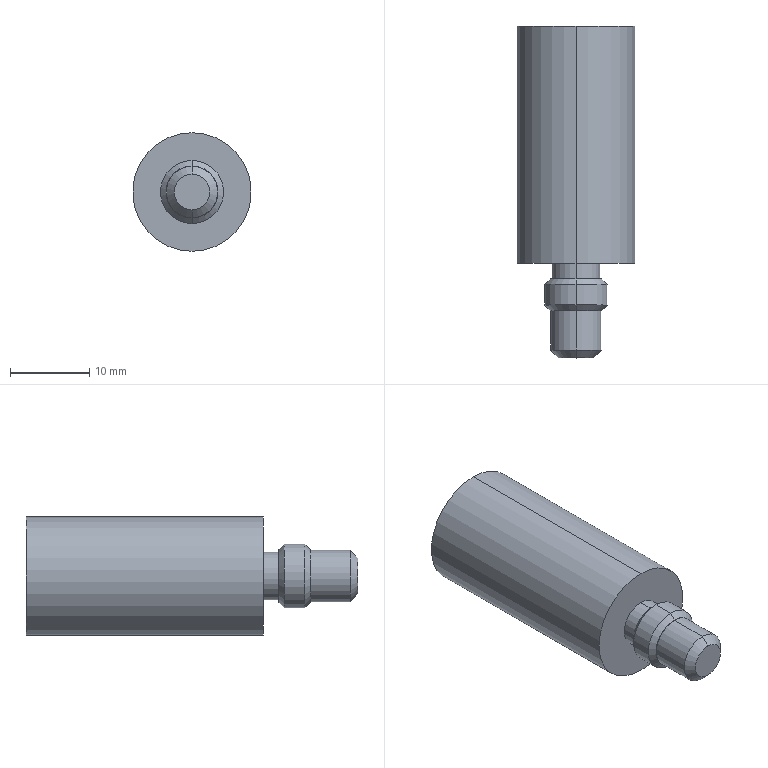Part | STEP file | X77-09213 | 1 solid | 25 faces | box 15 x 42 x 15 mm | volume 5004 mm3 | cone 10 | cylinder 10 | plane 5 | commonest cylinder face diameters 6.5 x4 6 x2 8 x2 15 x2
STEP:
#1=CARTESIAN_POINT('',(0.,40.,-3.25));
#2=VERTEX_POINT('',#1);
#3=CARTESIAN_POINT('',(0.,40.,3.25));
#4=VERTEX_POINT('',#3);
#5=CARTESIAN_POINT('',(0.,40.,0.));
#6=DIRECTION('',(0.,1.,0.));
#7=DIRECTION('',(0.,0.,-1.));
#8=AXIS2_PLACEMENT_3D('',#5,#6,#7);
#9=CIRCLE('',#8,3.25);
#10=EDGE_CURVE('',#2,#4,#9,.T.);
#11=ORIENTED_EDGE('',*,*,#10,.F.);
#12=CARTESIAN_POINT('',(0.,42.,-5.25));
#13=VERTEX_POINT('',#12);
#14=CARTESIAN_POINT('',(0.,42.,-5.25));
#15=DIRECTION('',(0.,0.7071,-0.7071));
#16=VECTOR('',#15,1000.);
#17=LINE('',#14,#16);
#18=EDGE_CURVE('',#2,#13,#17,.T.);
#19=ORIENTED_EDGE('',*,*,#18,.T.);
#20=CARTESIAN_POINT('',(0.,42.,5.25));
#21=VERTEX_POINT('',#20);
#22=CARTESIAN_POINT('',(0.,42.,0.));
#23=DIRECTION('',(0.,-1.,0.));
#24=DIRECTION('',(0.,0.,-1.));
#25=AXIS2_PLACEMENT_3D('',#22,#23,#24);
#26=CIRCLE('',#25,5.25);
#27=EDGE_CURVE('',#21,#13,#26,.T.);
#28=ORIENTED_EDGE('',*,*,#27,.F.);
#29=CARTESIAN_POINT('',(0.,42.,5.25));
#30=DIRECTION('',(0.,0.7071,0.7071));
#31=VECTOR('',#30,1000.);
#32=LINE('',#29,#31);
#33=EDGE_CURVE('',#4,#21,#32,.T.);
#34=ORIENTED_EDGE('',*,*,#33,.F.);
#35=EDGE_LOOP('',(#11,#19,#28,#34));
#36=FACE_OUTER_BOUND('',#35,.T.);
#37=CARTESIAN_POINT('',(0.,42.,0.));
#38=DIRECTION('',(0.,1.,0.));
#39=DIRECTION('',(0.,0.,1.));
#40=AXIS2_PLACEMENT_3D('',#37,#38,#39);
#41=CONICAL_SURFACE('',#40,5.25,0.7854);
#42=ADVANCED_FACE('',(#36),#41,.F.);
#43=CARTESIAN_POINT('',(0.,0.,-2.25));
#44=VERTEX_POINT('',#43);
#45=CARTESIAN_POINT('',(0.,0.,2.25));
#46=VERTEX_POINT('',#45);
#47=CARTESIAN_POINT('',(0.,0.,0.));
#48=DIRECTION('',(0.,-1.,0.));
#49=DIRECTION('',(0.,0.,-1.));
#50=AXIS2_PLACEMENT_3D('',#47,#48,#49);
#51=CIRCLE('',#50,2.25);
#52=EDGE_CURVE('',#44,#46,#51,.T.);
#53=ORIENTED_EDGE('',*,*,#52,.F.);
#54=CARTESIAN_POINT('',(0.,1.,-3.25));
#55=VERTEX_POINT('',#54);
#56=CARTESIAN_POINT('',(0.,1.,-3.25));
#57=DIRECTION('',(0.,0.7071,-0.7071));
#58=VECTOR('',#57,1000.);
#59=LINE('',#56,#58);
#60=EDGE_CURVE('',#44,#55,#59,.T.);
#61=ORIENTED_EDGE('',*,*,#60,.T.);
#62=CARTESIAN_POINT('',(0.,1.,3.25));
#63=VERTEX_POINT('',#62);
#64=CARTESIAN_POINT('',(0.,1.,0.));
#65=DIRECTION('',(0.,-1.,0.));
#66=DIRECTION('',(0.,0.,-1.));
#67=AXIS2_PLACEMENT_3D('',#64,#65,#66);
#68=CIRCLE('',#67,3.25);
#69=EDGE_CURVE('',#55,#63,#68,.T.);
#70=ORIENTED_EDGE('',*,*,#69,.T.);
#71=CARTESIAN_POINT('',(0.,1.,3.25));
#72=DIRECTION('',(0.,0.7071,0.7071));
#73=VECTOR('',#72,1000.);
#74=LINE('',#71,#73);
#75=EDGE_CURVE('',#46,#63,#74,.T.);
#76=ORIENTED_EDGE('',*,*,#75,.F.);
#77=EDGE_LOOP('',(#53,#61,#70,#76));
#78=FACE_OUTER_BOUND('',#77,.T.);
#79=CARTESIAN_POINT('',(0.,1.,0.));
#80=DIRECTION('',(0.,1.,0.));
#81=DIRECTION('',(0.,0.,1.));
#82=AXIS2_PLACEMENT_3D('',#79,#80,#81);
#83=CONICAL_SURFACE('',#82,3.25,0.7854);
#84=ADVANCED_FACE('',(#78),#83,.T.);
#85=CARTESIAN_POINT('',(0.,6.,-3.25));
#86=VERTEX_POINT('',#85);
#87=CARTESIAN_POINT('',(0.,6.,3.25));
#88=VERTEX_POINT('',#87);
#89=CARTESIAN_POINT('',(0.,6.,0.));
#90=DIRECTION('',(0.,-1.,0.));
#91=DIRECTION('',(0.,0.,-1.));
#92=AXIS2_PLACEMENT_3D('',#89,#90,#91);
#93=CIRCLE('',#92,3.25);
#94=EDGE_CURVE('',#86,#88,#93,.T.);
#95=ORIENTED_EDGE('',*,*,#94,.T.);
#96=CARTESIAN_POINT('',(0.,0.,3.25));
#97=DIRECTION('',(0.,-1.,0.));
#98=VECTOR('',#97,1000.);
#99=LINE('',#96,#98);
#100=EDGE_CURVE('',#88,#63,#99,.T.);
#101=ORIENTED_EDGE('',*,*,#100,.T.);
#102=ORIENTED_EDGE('',*,*,#69,.F.);
#103=CARTESIAN_POINT('',(0.,0.,-3.25));
#104=DIRECTION('',(0.,-1.,0.));
#105=VECTOR('',#104,1000.);
#106=LINE('',#103,#105);
#107=EDGE_CURVE('',#86,#55,#106,.T.);
#108=ORIENTED_EDGE('',*,*,#107,.F.);
#109=EDGE_LOOP('',(#95,#101,#102,#108));
#110=FACE_OUTER_BOUND('',#109,.T.);
#111=CARTESIAN_POINT('',(0.,0.,0.));
#112=DIRECTION('',(0.,-1.,0.));
#113=DIRECTION('',(0.,0.,-1.));
#114=AXIS2_PLACEMENT_3D('',#111,#112,#113);
#115=CYLINDRICAL_SURFACE('',#114,3.25);
#116=ADVANCED_FACE('',(#110),#115,.T.);
#117=CARTESIAN_POINT('',(0.,6.,-3.3));
#118=VERTEX_POINT('',#117);
#119=CARTESIAN_POINT('',(0.,6.,3.3));
#120=VERTEX_POINT('',#119);
#121=CARTESIAN_POINT('',(0.,6.,0.));
#122=DIRECTION('',(0.,-1.,0.));
#123=DIRECTION('',(0.,0.,-1.));
#124=AXIS2_PLACEMENT_3D('',#121,#122,#123);
#125=CIRCLE('',#124,3.3);
#126=EDGE_CURVE('',#118,#120,#125,.T.);
#127=ORIENTED_EDGE('',*,*,#126,.F.);
#128=CARTESIAN_POINT('',(0.,6.7,-4.));
#129=VERTEX_POINT('',#128);
#130=CARTESIAN_POINT('',(0.,6.7,-4.));
#131=DIRECTION('',(0.,0.7071,-0.7071));
#132=VECTOR('',#131,1000.);
#133=LINE('',#130,#132);
#134=EDGE_CURVE('',#118,#129,#133,.T.);
#135=ORIENTED_EDGE('',*,*,#134,.T.);
#136=CARTESIAN_POINT('',(0.,6.7,4.));
#137=VERTEX_POINT('',#136);
#138=CARTESIAN_POINT('',(0.,6.7,0.));
#139=DIRECTION('',(0.,-1.,0.));
#140=DIRECTION('',(0.,0.,-1.));
#141=AXIS2_PLACEMENT_3D('',#138,#139,#140);
#142=CIRCLE('',#141,4.);
#143=EDGE_CURVE('',#129,#137,#142,.T.);
#144=ORIENTED_EDGE('',*,*,#143,.T.);
#145=CARTESIAN_POINT('',(0.,6.7,4.));
#146=DIRECTION('',(0.,0.7071,0.7071));
#147=VECTOR('',#146,1000.);
#148=LINE('',#145,#147);
#149=EDGE_CURVE('',#120,#137,#148,.T.);
#150=ORIENTED_EDGE('',*,*,#149,.F.);
#151=EDGE_LOOP('',(#127,#135,#144,#150));
#152=FACE_OUTER_BOUND('',#151,.T.);
#153=CARTESIAN_POINT('',(0.,6.7,0.));
#154=DIRECTION('',(0.,1.,0.));
#155=DIRECTION('',(0.,0.,1.));
#156=AXIS2_PLACEMENT_3D('',#153,#154,#155);
#157=CONICAL_SURFACE('',#156,4.,0.7854);
#158=ADVANCED_FACE('',(#152),#157,.T.);
#159=CARTESIAN_POINT('',(0.,9.3,-4.));
#160=VERTEX_POINT('',#159);
#161=CARTESIAN_POINT('',(0.,9.3,4.));
#162=VERTEX_POINT('',#161);
#163=CARTESIAN_POINT('',(0.,9.3,0.));
#164=DIRECTION('',(0.,-1.,0.));
#165=DIRECTION('',(0.,0.,-1.));
#166=AXIS2_PLACEMENT_3D('',#163,#164,#165);
#167=CIRCLE('',#166,4.);
#168=EDGE_CURVE('',#160,#162,#167,.T.);
#169=ORIENTED_EDGE('',*,*,#168,.T.);
#170=CARTESIAN_POINT('',(0.,0.,4.));
#171=DIRECTION('',(0.,-1.,0.));
#172=VECTOR('',#171,1000.);
#173=LINE('',#170,#172);
#174=EDGE_CURVE('',#162,#137,#173,.T.);
#175=ORIENTED_EDGE('',*,*,#174,.T.);
#176=ORIENTED_EDGE('',*,*,#143,.F.);
#177=CARTESIAN_POINT('',(0.,0.,-4.));
#178=DIRECTION('',(0.,-1.,0.));
#179=VECTOR('',#178,1000.);
#180=LINE('',#177,#179);
#181=EDGE_CURVE('',#160,#129,#180,.T.);
#182=ORIENTED_EDGE('',*,*,#181,.F.);
#183=EDGE_LOOP('',(#169,#175,#176,#182));
#184=FACE_OUTER_BOUND('',#183,.T.);
#185=CARTESIAN_POINT('',(0.,0.,0.));
#186=DIRECTION('',(0.,-1.,0.));
#187=DIRECTION('',(0.,0.,-1.));
#188=AXIS2_PLACEMENT_3D('',#185,#186,#187);
#189=CYLINDRICAL_SURFACE('',#188,4.);
#190=ADVANCED_FACE('',(#184),#189,.T.);
#191=CARTESIAN_POINT('',(0.,10.,-3.3));
#192=VERTEX_POINT('',#191);
#193=CARTESIAN_POINT('',(0.,10.,3.3));
#194=VERTEX_POINT('',#193);
#195=CARTESIAN_POINT('',(0.,10.,0.));
#196=DIRECTION('',(0.,-1.,0.));
#197=DIRECTION('',(0.,0.,-1.));
#198=AXIS2_PLACEMENT_3D('',#195,#196,#197);
#199=CIRCLE('',#198,3.3);
#200=EDGE_CURVE('',#192,#194,#199,.T.);
#201=ORIENTED_EDGE('',*,*,#200,.T.);
#202=CARTESIAN_POINT('',(0.,10.,3.3));
#203=DIRECTION('',(0.,-0.7071,0.7071));
#204=VECTOR('',#203,1000.);
#205=LINE('',#202,#204);
#206=EDGE_CURVE('',#194,#162,#205,.T.);
#207=ORIENTED_EDGE('',*,*,#206,.T.);
#208=ORIENTED_EDGE('',*,*,#168,.F.);
#209=CARTESIAN_POINT('',(0.,10.,-3.3));
#210=DIRECTION('',(0.,-0.7071,-0.7071));
#211=VECTOR('',#210,1000.);
#212=LINE('',#209,#211);
#213=EDGE_CURVE('',#192,#160,#212,.T.);
#214=ORIENTED_EDGE('',*,*,#213,.F.);
#215=EDGE_LOOP('',(#201,#207,#208,#214));
#216=FACE_OUTER_BOUND('',#215,.T.);
#217=CARTESIAN_POINT('',(0.,10.,0.));
#218=DIRECTION('',(0.,-1.,0.));
#219=DIRECTION('',(0.,0.,-1.));
#220=AXIS2_PLACEMENT_3D('',#217,#218,#219);
#221=CONICAL_SURFACE('',#220,3.3,0.7854);
#222=ADVANCED_FACE('',(#216),#221,.T.);
#223=CARTESIAN_POINT('',(0.,12.,-3.));
#224=VERTEX_POINT('',#223);
#225=CARTESIAN_POINT('',(0.,12.,3.));
#226=VERTEX_POINT('',#225);
#227=CARTESIAN_POINT('',(0.,12.,0.));
#228=DIRECTION('',(0.,-1.,0.));
#229=DIRECTION('',(0.,0.,-1.));
#230=AXIS2_PLACEMENT_3D('',#227,#228,#229);
#231=CIRCLE('',#230,3.);
#232=EDGE_CURVE('',#224,#226,#231,.T.);
#233=ORIENTED_EDGE('',*,*,#232,.T.);
#234=CARTESIAN_POINT('',(0.,10.,3.));
#235=VERTEX_POINT('',#234);
#236=CARTESIAN_POINT('',(0.,0.,3.));
#237=DIRECTION('',(0.,-1.,0.));
#238=VECTOR('',#237,1000.);
#239=LINE('',#236,#238);
#240=EDGE_CURVE('',#226,#235,#239,.T.);
#241=ORIENTED_EDGE('',*,*,#240,.T.);
#242=CARTESIAN_POINT('',(0.,10.,-3.));
#243=VERTEX_POINT('',#242);
#244=CARTESIAN_POINT('',(0.,10.,0.));
#245=DIRECTION('',(0.,-1.,0.));
#246=DIRECTION('',(0.,0.,-1.));
#247=AXIS2_PLACEMENT_3D('',#244,#245,#246);
#248=CIRCLE('',#247,3.);
#249=EDGE_CURVE('',#243,#235,#248,.T.);
#250=ORIENTED_EDGE('',*,*,#249,.F.);
#251=CARTESIAN_POINT('',(0.,0.,-3.));
#252=DIRECTION('',(0.,-1.,0.));
#253=VECTOR('',#252,1000.);
#254=LINE('',#251,#253);
#255=EDGE_CURVE('',#224,#243,#254,.T.);
#256=ORIENTED_EDGE('',*,*,#255,.F.);
#257=EDGE_LOOP('',(#233,#241,#250,#256));
#258=FACE_OUTER_BOUND('',#257,.T.);
#259=CARTESIAN_POINT('',(0.,0.,0.));
#260=DIRECTION('',(0.,-1.,0.));
#261=DIRECTION('',(0.,0.,-1.));
#262=AXIS2_PLACEMENT_3D('',#259,#260,#261);
#263=CYLINDRICAL_SURFACE('',#262,3.);
#264=ADVANCED_FACE('',(#258),#263,.T.);
#265=CARTESIAN_POINT('',(0.,42.,-7.5));
#266=VERTEX_POINT('',#265);
#267=CARTESIAN_POINT('',(0.,42.,7.5));
#268=VERTEX_POINT('',#267);
#269=CARTESIAN_POINT('',(0.,42.,0.));
#270=DIRECTION('',(0.,-1.,0.));
#271=DIRECTION('',(0.,0.,-1.));
#272=AXIS2_PLACEMENT_3D('',#269,#270,#271);
#273=CIRCLE('',#272,7.5);
#274=EDGE_CURVE('',#266,#268,#273,.T.);
#275=ORIENTED_EDGE('',*,*,#274,.T.);
#276=CARTESIAN_POINT('',(0.,12.,7.5));
#277=VERTEX_POINT('',#276);
#278=CARTESIAN_POINT('',(0.,0.,7.5));
#279=DIRECTION('',(0.,-1.,0.));
#280=VECTOR('',#279,1000.);
#281=LINE('',#278,#280);
#282=EDGE_CURVE('',#268,#277,#281,.T.);
#283=ORIENTED_EDGE('',*,*,#282,.T.);
#284=CARTESIAN_POINT('',(0.,12.,-7.5));
#285=VERTEX_POINT('',#284);
#286=CARTESIAN_POINT('',(0.,12.,0.));
#287=DIRECTION('',(0.,-1.,0.));
#288=DIRECTION('',(0.,0.,-1.));
#289=AXIS2_PLACEMENT_3D('',#286,#287,#288);
#290=CIRCLE('',#289,7.5);
#291=EDGE_CURVE('',#285,#277,#290,.T.);
#292=ORIENTED_EDGE('',*,*,#291,.F.);
#293=CARTESIAN_POINT('',(0.,0.,-7.5));
#294=DIRECTION('',(0.,-1.,0.));
#295=VECTOR('',#294,1000.);
#296=LINE('',#293,#295);
#297=EDGE_CURVE('',#266,#285,#296,.T.);
#298=ORIENTED_EDGE('',*,*,#297,.F.);
#299=EDGE_LOOP('',(#275,#283,#292,#298));
#300=FACE_OUTER_BOUND('',#299,.T.);
#301=CARTESIAN_POINT('',(0.,0.,0.));
#302=DIRECTION('',(0.,-1.,0.));
#303=DIRECTION('',(0.,0.,-1.));
#304=AXIS2_PLACEMENT_3D('',#301,#302,#303);
#305=CYLINDRICAL_SURFACE('',#304,7.5);
#306=ADVANCED_FACE('',(#300),#305,.T.);
#307=ORIENTED_EDGE('',*,*,#10,.T.);
#308=CARTESIAN_POINT('',(0.,22.,3.25));
#309=VERTEX_POINT('',#308);
#310=CARTESIAN_POINT('',(0.,0.,3.25));
#311=DIRECTION('',(0.,-1.,0.));
#312=VECTOR('',#311,1000.);
#313=LINE('',#310,#312);
#314=EDGE_CURVE('',#4,#309,#313,.T.);
#315=ORIENTED_EDGE('',*,*,#314,.T.);
#316=CARTESIAN_POINT('',(0.,22.,-3.25));
#317=VERTEX_POINT('',#316);
#318=CARTESIAN_POINT('',(0.,22.,0.));
#319=DIRECTION('',(0.,-1.,0.));
#320=DIRECTION('',(0.,0.,-1.));
#321=AXIS2_PLACEMENT_3D('',#318,#319,#320);
#322=CIRCLE('',#321,3.25);
#323=EDGE_CURVE('',#309,#317,#322,.T.);
#324=ORIENTED_EDGE('',*,*,#323,.T.);
#325=CARTESIAN_POINT('',(0.,0.,-3.25));
#326=DIRECTION('',(0.,-1.,0.));
#327=VECTOR('',#326,1000.);
#328=LINE('',#325,#327);
#329=EDGE_CURVE('',#2,#317,#328,.T.);
#330=ORIENTED_EDGE('',*,*,#329,.F.);
#331=EDGE_LOOP('',(#307,#315,#324,#330));
#332=FACE_OUTER_BOUND('',#331,.T.);
#333=CARTESIAN_POINT('',(0.,0.,0.));
#334=DIRECTION('',(0.,-1.,0.));
#335=DIRECTION('',(0.,0.,-1.));
#336=AXIS2_PLACEMENT_3D('',#333,#334,#335);
#337=CYLINDRICAL_SURFACE('',#336,3.25);
#338=ADVANCED_FACE('',(#332),#337,.F.);
#339=CARTESIAN_POINT('',(0.,20.124,0.));
#340=VERTEX_POINT('',#339);
#341=CARTESIAN_POINT('',(0.,20.124,0.));
#342=DIRECTION('',(0.,0.5,0.866));
#343=VECTOR('',#342,1000.);
#344=LINE('',#341,#343);
#345=EDGE_CURVE('',#340,#309,#344,.T.);
#346=ORIENTED_EDGE('',*,*,#345,.F.);
#347=CARTESIAN_POINT('',(0.,20.124,0.));
#348=DIRECTION('',(0.,0.5,-0.866));
#349=VECTOR('',#348,1000.);
#350=LINE('',#347,#349);
#351=EDGE_CURVE('',#340,#317,#350,.T.);
#352=ORIENTED_EDGE('',*,*,#351,.T.);
#353=ORIENTED_EDGE('',*,*,#323,.F.);
#354=EDGE_LOOP('',(#346,#352,#353));
#355=FACE_OUTER_BOUND('',#354,.T.);
#356=CARTESIAN_POINT('',(0.,1020.124,0.));
#357=DIRECTION('',(0.,1.,0.));
#358=DIRECTION('',(0.,0.,1.));
#359=AXIS2_PLACEMENT_3D('',#356,#357,#358);
#360=CONICAL_SURFACE('',#359,1732.051,1.047);
#361=ADVANCED_FACE('',(#355),#360,.F.);
#362=ORIENTED_EDGE('',*,*,#351,.F.);
#363=ORIENTED_EDGE('',*,*,#345,.T.);
#364=CARTESIAN_POINT('',(0.,22.,0.));
#365=DIRECTION('',(0.,-1.,0.));
#366=DIRECTION('',(0.,0.,-1.));
#367=AXIS2_PLACEMENT_3D('',#364,#365,#366);
#368=CIRCLE('',#367,3.25);
#369=EDGE_CURVE('',#317,#309,#368,.T.);
#370=ORIENTED_EDGE('',*,*,#369,.F.);
#371=EDGE_LOOP('',(#362,#363,#370));
#372=FACE_OUTER_BOUND('',#371,.T.);
#373=CARTESIAN_POINT('',(0.,1020.124,0.));
#374=DIRECTION('',(0.,1.,0.));
#375=DIRECTION('',(0.,0.,1.));
#376=AXIS2_PLACEMENT_3D('',#373,#374,#375);
#377=CONICAL_SURFACE('',#376,1732.051,1.047);
#378=ADVANCED_FACE('',(#372),#377,.F.);
#379=ORIENTED_EDGE('',*,*,#314,.F.);
#380=CARTESIAN_POINT('',(0.,40.,0.));
#381=DIRECTION('',(0.,1.,0.));
#382=DIRECTION('',(0.,0.,-1.));
#383=AXIS2_PLACEMENT_3D('',#380,#381,#382);
#384=CIRCLE('',#383,3.25);
#385=EDGE_CURVE('',#4,#2,#384,.T.);
#386=ORIENTED_EDGE('',*,*,#385,.T.);
#387=ORIENTED_EDGE('',*,*,#329,.T.);
#388=ORIENTED_EDGE('',*,*,#369,.T.);
#389=EDGE_LOOP('',(#379,#386,#387,#388));
#390=FACE_OUTER_BOUND('',#389,.T.);
#391=CARTESIAN_POINT('',(0.,0.,0.));
#392=DIRECTION('',(0.,-1.,0.));
#393=DIRECTION('',(0.,0.,-1.));
#394=AXIS2_PLACEMENT_3D('',#391,#392,#393);
#395=CYLINDRICAL_SURFACE('',#394,3.25);
#396=ADVANCED_FACE('',(#390),#395,.F.);
#397=ORIENTED_EDGE('',*,*,#27,.T.);
#398=CARTESIAN_POINT('',(0.,42.,0.));
#399=DIRECTION('',(0.,-1.,0.));
#400=DIRECTION('',(0.,0.,-1.));
#401=AXIS2_PLACEMENT_3D('',#398,#399,#400);
#402=CIRCLE('',#401,5.25);
#403=EDGE_CURVE('',#13,#21,#402,.T.);
#404=ORIENTED_EDGE('',*,*,#403,.T.);
#405=EDGE_LOOP('',(#397,#404));
#406=FACE_BOUND('',#405,.T.);
#407=ORIENTED_EDGE('',*,*,#274,.F.);
#408=CARTESIAN_POINT('',(0.,42.,0.));
#409=DIRECTION('',(0.,-1.,0.));
#410=DIRECTION('',(0.,0.,-1.));
#411=AXIS2_PLACEMENT_3D('',#408,#409,#410);
#412=CIRCLE('',#411,7.5);
#413=EDGE_CURVE('',#268,#266,#412,.T.);
#414=ORIENTED_EDGE('',*,*,#413,.F.);
#415=EDGE_LOOP('',(#407,#414));
#416=FACE_OUTER_BOUND('',#415,.T.);
#417=CARTESIAN_POINT('',(-3.25,42.,0.));
#418=DIRECTION('',(0.,-1.,0.));
#419=DIRECTION('',(0.,0.,-1.));
#420=AXIS2_PLACEMENT_3D('',#417,#418,#419);
#421=PLANE('',#420);
#422=ADVANCED_FACE('',(#406,#416),#421,.F.);
#423=ORIENTED_EDGE('',*,*,#282,.F.);
#424=ORIENTED_EDGE('',*,*,#413,.T.);
#425=ORIENTED_EDGE('',*,*,#297,.T.);
#426=CARTESIAN_POINT('',(0.,12.,0.));
#427=DIRECTION('',(0.,-1.,0.));
#428=DIRECTION('',(0.,0.,-1.));
#429=AXIS2_PLACEMENT_3D('',#426,#427,#428);
#430=CIRCLE('',#429,7.5);
#431=EDGE_CURVE('',#277,#285,#430,.T.);
#432=ORIENTED_EDGE('',*,*,#431,.F.);
#433=EDGE_LOOP('',(#423,#424,#425,#432));
#434=FACE_OUTER_BOUND('',#433,.T.);
#435=CARTESIAN_POINT('',(0.,0.,0.));
#436=DIRECTION('',(0.,-1.,0.));
#437=DIRECTION('',(0.,0.,-1.));
#438=AXIS2_PLACEMENT_3D('',#435,#436,#437);
#439=CYLINDRICAL_SURFACE('',#438,7.5);
#440=ADVANCED_FACE('',(#434),#439,.T.);
#441=ORIENTED_EDGE('',*,*,#232,.F.);
#442=CARTESIAN_POINT('',(0.,12.,0.));
#443=DIRECTION('',(0.,-1.,0.));
#444=DIRECTION('',(0.,0.,-1.));
#445=AXIS2_PLACEMENT_3D('',#442,#443,#444);
#446=CIRCLE('',#445,3.);
#447=EDGE_CURVE('',#226,#224,#446,.T.);
#448=ORIENTED_EDGE('',*,*,#447,.F.);
#449=EDGE_LOOP('',(#441,#448));
#450=FACE_BOUND('',#449,.T.);
#451=ORIENTED_EDGE('',*,*,#291,.T.);
#452=ORIENTED_EDGE('',*,*,#431,.T.);
#453=EDGE_LOOP('',(#451,#452));
#454=FACE_OUTER_BOUND('',#453,.T.);
#455=CARTESIAN_POINT('',(-4.,12.,0.));
#456=DIRECTION('',(0.,1.,0.));
#457=DIRECTION('',(0.,0.,1.));
#458=AXIS2_PLACEMENT_3D('',#455,#456,#457);
#459=PLANE('',#458);
#460=ADVANCED_FACE('',(#450,#454),#459,.F.);
#461=ORIENTED_EDGE('',*,*,#240,.F.);
#462=ORIENTED_EDGE('',*,*,#447,.T.);
#463=ORIENTED_EDGE('',*,*,#255,.T.);
#464=CARTESIAN_POINT('',(0.,10.,0.));
#465=DIRECTION('',(0.,-1.,0.));
#466=DIRECTION('',(0.,0.,-1.));
#467=AXIS2_PLACEMENT_3D('',#464,#465,#466);
#468=CIRCLE('',#467,3.);
#469=EDGE_CURVE('',#235,#243,#468,.T.);
#470=ORIENTED_EDGE('',*,*,#469,.F.);
#471=EDGE_LOOP('',(#461,#462,#463,#470));
#472=FACE_OUTER_BOUND('',#471,.T.);
#473=CARTESIAN_POINT('',(0.,0.,0.));
#474=DIRECTION('',(0.,-1.,0.));
#475=DIRECTION('',(0.,0.,-1.));
#476=AXIS2_PLACEMENT_3D('',#473,#474,#475);
#477=CYLINDRICAL_SURFACE('',#476,3.);
#478=ADVANCED_FACE('',(#472),#477,.T.);
#479=ORIENTED_EDGE('',*,*,#200,.F.);
#480=CARTESIAN_POINT('',(0.,10.,0.));
#481=DIRECTION('',(0.,-1.,0.));
#482=DIRECTION('',(0.,0.,-1.));
#483=AXIS2_PLACEMENT_3D('',#480,#481,#482);
#484=CIRCLE('',#483,3.3);
#485=EDGE_CURVE('',#194,#192,#484,.T.);
#486=ORIENTED_EDGE('',*,*,#485,.F.);
#487=EDGE_LOOP('',(#479,#486));
#488=FACE_OUTER_BOUND('',#487,.T.);
#489=ORIENTED_EDGE('',*,*,#249,.T.);
#490=ORIENTED_EDGE('',*,*,#469,.T.);
#491=EDGE_LOOP('',(#489,#490));
#492=FACE_BOUND('',#491,.T.);
#493=CARTESIAN_POINT('',(-3.3,10.,0.));
#494=DIRECTION('',(0.,-1.,0.));
#495=DIRECTION('',(0.,0.,-1.));
#496=AXIS2_PLACEMENT_3D('',#493,#494,#495);
#497=PLANE('',#496);
#498=ADVANCED_FACE('',(#488,#492),#497,.F.);
#499=ORIENTED_EDGE('',*,*,#206,.F.);
#500=ORIENTED_EDGE('',*,*,#485,.T.);
#501=ORIENTED_EDGE('',*,*,#213,.T.);
#502=CARTESIAN_POINT('',(0.,9.3,0.));
#503=DIRECTION('',(0.,-1.,0.));
#504=DIRECTION('',(0.,0.,-1.));
#505=AXIS2_PLACEMENT_3D('',#502,#503,#504);
#506=CIRCLE('',#505,4.);
#507=EDGE_CURVE('',#162,#160,#506,.T.);
#508=ORIENTED_EDGE('',*,*,#507,.F.);
#509=EDGE_LOOP('',(#499,#500,#501,#508));
#510=FACE_OUTER_BOUND('',#509,.T.);
#511=CARTESIAN_POINT('',(0.,10.,0.));
#512=DIRECTION('',(0.,-1.,0.));
#513=DIRECTION('',(0.,0.,-1.));
#514=AXIS2_PLACEMENT_3D('',#511,#512,#513);
#515=CONICAL_SURFACE('',#514,3.3,0.7854);
#516=ADVANCED_FACE('',(#510),#515,.T.);
#517=ORIENTED_EDGE('',*,*,#174,.F.);
#518=ORIENTED_EDGE('',*,*,#507,.T.);
#519=ORIENTED_EDGE('',*,*,#181,.T.);
#520=CARTESIAN_POINT('',(0.,6.7,0.));
#521=DIRECTION('',(0.,-1.,0.));
#522=DIRECTION('',(0.,0.,-1.));
#523=AXIS2_PLACEMENT_3D('',#520,#521,#522);
#524=CIRCLE('',#523,4.);
#525=EDGE_CURVE('',#137,#129,#524,.T.);
#526=ORIENTED_EDGE('',*,*,#525,.F.);
#527=EDGE_LOOP('',(#517,#518,#519,#526));
#528=FACE_OUTER_BOUND('',#527,.T.);
#529=CARTESIAN_POINT('',(0.,0.,0.));
#530=DIRECTION('',(0.,-1.,0.));
#531=DIRECTION('',(0.,0.,-1.));
#532=AXIS2_PLACEMENT_3D('',#529,#530,#531);
#533=CYLINDRICAL_SURFACE('',#532,4.);
#534=ADVANCED_FACE('',(#528),#533,.T.);
#535=ORIENTED_EDGE('',*,*,#134,.F.);
#536=CARTESIAN_POINT('',(0.,6.,0.));
#537=DIRECTION('',(0.,-1.,0.));
#538=DIRECTION('',(0.,0.,-1.));
#539=AXIS2_PLACEMENT_3D('',#536,#537,#538);
#540=CIRCLE('',#539,3.3);
#541=EDGE_CURVE('',#120,#118,#540,.T.);
#542=ORIENTED_EDGE('',*,*,#541,.F.);
#543=ORIENTED_EDGE('',*,*,#149,.T.);
#544=ORIENTED_EDGE('',*,*,#525,.T.);
#545=EDGE_LOOP('',(#535,#542,#543,#544));
#546=FACE_OUTER_BOUND('',#545,.T.);
#547=CARTESIAN_POINT('',(0.,6.7,0.));
#548=DIRECTION('',(0.,1.,0.));
#549=DIRECTION('',(0.,0.,1.));
#550=AXIS2_PLACEMENT_3D('',#547,#548,#549);
#551=CONICAL_SURFACE('',#550,4.,0.7854);
#552=ADVANCED_FACE('',(#546),#551,.T.);
#553=ORIENTED_EDGE('',*,*,#94,.F.);
#554=CARTESIAN_POINT('',(0.,6.,0.));
#555=DIRECTION('',(0.,-1.,0.));
#556=DIRECTION('',(0.,0.,-1.));
#557=AXIS2_PLACEMENT_3D('',#554,#555,#556);
#558=CIRCLE('',#557,3.25);
#559=EDGE_CURVE('',#88,#86,#558,.T.);
#560=ORIENTED_EDGE('',*,*,#559,.F.);
#561=EDGE_LOOP('',(#553,#560));
#562=FACE_BOUND('',#561,.T.);
#563=ORIENTED_EDGE('',*,*,#541,.T.);
#564=ORIENTED_EDGE('',*,*,#126,.T.);
#565=EDGE_LOOP('',(#563,#564));
#566=FACE_OUTER_BOUND('',#565,.T.);
#567=CARTESIAN_POINT('',(-3.25,6.,0.));
#568=DIRECTION('',(0.,1.,0.));
#569=DIRECTION('',(0.,0.,1.));
#570=AXIS2_PLACEMENT_3D('',#567,#568,#569);
#571=PLANE('',#570);
#572=ADVANCED_FACE('',(#562,#566),#571,.F.);
#573=ORIENTED_EDGE('',*,*,#100,.F.);
#574=ORIENTED_EDGE('',*,*,#559,.T.);
#575=ORIENTED_EDGE('',*,*,#107,.T.);
#576=CARTESIAN_POINT('',(0.,1.,0.));
#577=DIRECTION('',(0.,-1.,0.));
#578=DIRECTION('',(0.,0.,-1.));
#579=AXIS2_PLACEMENT_3D('',#576,#577,#578);
#580=CIRCLE('',#579,3.25);
#581=EDGE_CURVE('',#63,#55,#580,.T.);
#582=ORIENTED_EDGE('',*,*,#581,.F.);
#583=EDGE_LOOP('',(#573,#574,#575,#582));
#584=FACE_OUTER_BOUND('',#583,.T.);
#585=CARTESIAN_POINT('',(0.,0.,0.));
#586=DIRECTION('',(0.,-1.,0.));
#587=DIRECTION('',(0.,0.,-1.));
#588=AXIS2_PLACEMENT_3D('',#585,#586,#587);
#589=CYLINDRICAL_SURFACE('',#588,3.25);
#590=ADVANCED_FACE('',(#584),#589,.T.);
#591=ORIENTED_EDGE('',*,*,#60,.F.);
#592=CARTESIAN_POINT('',(0.,0.,0.));
#593=DIRECTION('',(0.,-1.,0.));
#594=DIRECTION('',(0.,0.,-1.));
#595=AXIS2_PLACEMENT_3D('',#592,#593,#594);
#596=CIRCLE('',#595,2.25);
#597=EDGE_CURVE('',#46,#44,#596,.T.);
#598=ORIENTED_EDGE('',*,*,#597,.F.);
#599=ORIENTED_EDGE('',*,*,#75,.T.);
#600=ORIENTED_EDGE('',*,*,#581,.T.);
#601=EDGE_LOOP('',(#591,#598,#599,#600));
#602=FACE_OUTER_BOUND('',#601,.T.);
#603=CARTESIAN_POINT('',(0.,1.,0.));
#604=DIRECTION('',(0.,1.,0.));
#605=DIRECTION('',(0.,0.,1.));
#606=AXIS2_PLACEMENT_3D('',#603,#604,#605);
#607=CONICAL_SURFACE('',#606,3.25,0.7854);
#608=ADVANCED_FACE('',(#602),#607,.T.);
#609=ORIENTED_EDGE('',*,*,#597,.T.);
#610=ORIENTED_EDGE('',*,*,#52,.T.);
#611=EDGE_LOOP('',(#609,#610));
#612=FACE_OUTER_BOUND('',#611,.T.);
#613=CARTESIAN_POINT('',(-2.25,0.,0.));
#614=DIRECTION('',(0.,1.,0.));
#615=DIRECTION('',(0.,0.,1.));
#616=AXIS2_PLACEMENT_3D('',#613,#614,#615);
#617=PLANE('',#616);
#618=ADVANCED_FACE('',(#612),#617,.F.);
#619=ORIENTED_EDGE('',*,*,#18,.F.);
#620=ORIENTED_EDGE('',*,*,#385,.F.);
#621=ORIENTED_EDGE('',*,*,#33,.T.);
#622=ORIENTED_EDGE('',*,*,#403,.F.);
#623=EDGE_LOOP('',(#619,#620,#621,#622));
#624=FACE_OUTER_BOUND('',#623,.T.);
#625=CARTESIAN_POINT('',(0.,42.,0.));
#626=DIRECTION('',(0.,1.,0.));
#627=DIRECTION('',(0.,0.,1.));
#628=AXIS2_PLACEMENT_3D('',#625,#626,#627);
#629=CONICAL_SURFACE('',#628,5.25,0.7854);
#630=ADVANCED_FACE('',(#624),#629,.F.);
#631=CLOSED_SHELL('',(#42,#84,#116,#158,#190,#222,#264,#306,#338,#361,#378,#396,#422,#440,#460,#478,#498,#516,#534,#552,#572,#590,#608,#618,#630));
#632=MANIFOLD_SOLID_BREP('',#631);
#633=CARTESIAN_POINT('',(0.,0.,0.));
#634=DIRECTION('',(0.,0.,1.));
#635=DIRECTION('',(1.,0.,0.));
#636=AXIS2_PLACEMENT_3D('',#633,#634,#635);
#637=(LENGTH_UNIT()NAMED_UNIT(*)SI_UNIT(.MILLI.,.METRE.));
#638=UNCERTAINTY_MEASURE_WITH_UNIT(LENGTH_MEASURE(0.00001),#637,'','');
#639=(NAMED_UNIT(*)PLANE_ANGLE_UNIT()SI_UNIT($,.RADIAN.));
#640=(NAMED_UNIT(*)SI_UNIT($,.STERADIAN.)SOLID_ANGLE_UNIT());
#641=(GEOMETRIC_REPRESENTATION_CONTEXT(3)GLOBAL_UNCERTAINTY_ASSIGNED_CONTEXT((#638))GLOBAL_UNIT_ASSIGNED_CONTEXT((#637,#639,#640))REPRESENTATION_CONTEXT('',''));
#642=ADVANCED_BREP_SHAPE_REPRESENTATION('',(#632,#636),#641);